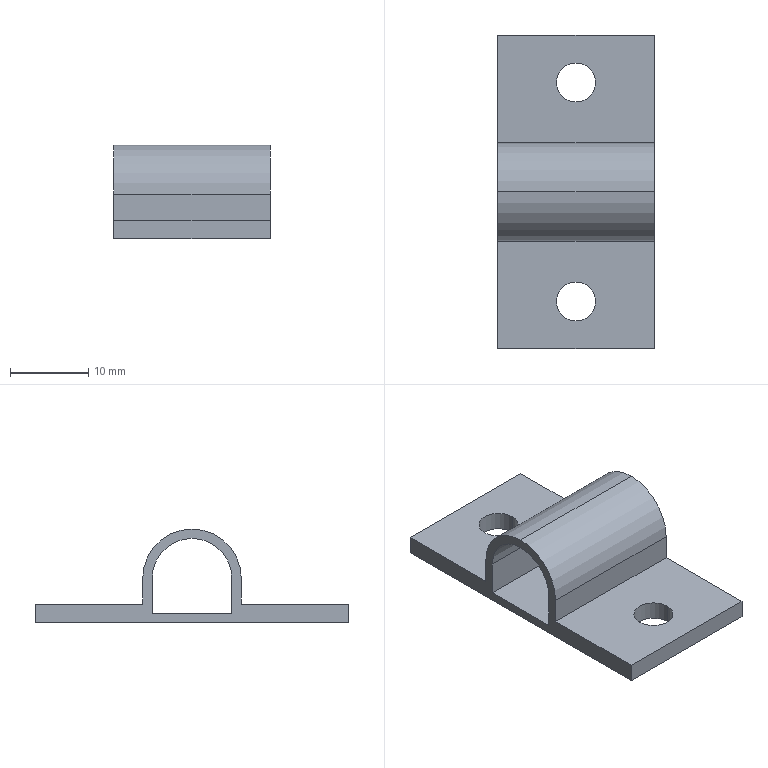Part | SolidWorks | features BaseBody 1 | 1 solid | 20 faces | box 20 x 40 x 12 mm | volume 2169 mm3 | plane 12 | cylinder 8 | commonest cylinder face diameters 5 x4 10.2 x2 12.6 x2
STEP:
#1=CARTESIAN_POINT('',(-7.5,14.,2.4));
#2=VERTEX_POINT('',#1);
#3=CARTESIAN_POINT('',(-12.5,14.,2.4));
#4=VERTEX_POINT('',#3);
#5=CARTESIAN_POINT('',(-10.,14.,2.4));
#6=DIRECTION('',(0.,0.,-1.));
#7=DIRECTION('',(-1.,0.,0.));
#8=AXIS2_PLACEMENT_3D('',#5,#6,#7);
#9=CIRCLE('',#8,2.5);
#10=EDGE_CURVE('',#2,#4,#9,.T.);
#11=ORIENTED_EDGE('',*,*,#10,.F.);
#12=CARTESIAN_POINT('',(-7.5,14.,0.));
#13=VERTEX_POINT('',#12);
#14=CARTESIAN_POINT('',(-7.5,14.,0.));
#15=DIRECTION('',(0.,0.,-1.));
#16=VECTOR('',#15,1000.);
#17=LINE('',#14,#16);
#18=EDGE_CURVE('',#2,#13,#17,.T.);
#19=ORIENTED_EDGE('',*,*,#18,.T.);
#20=CARTESIAN_POINT('',(-12.5,14.,0.));
#21=VERTEX_POINT('',#20);
#22=CARTESIAN_POINT('',(-10.,14.,0.));
#23=DIRECTION('',(0.,0.,1.));
#24=DIRECTION('',(-1.,0.,0.));
#25=AXIS2_PLACEMENT_3D('',#22,#23,#24);
#26=CIRCLE('',#25,2.5);
#27=EDGE_CURVE('',#21,#13,#26,.T.);
#28=ORIENTED_EDGE('',*,*,#27,.F.);
#29=CARTESIAN_POINT('',(-12.5,14.,0.));
#30=DIRECTION('',(0.,0.,-1.));
#31=VECTOR('',#30,1000.);
#32=LINE('',#29,#31);
#33=EDGE_CURVE('',#4,#21,#32,.T.);
#34=ORIENTED_EDGE('',*,*,#33,.F.);
#35=EDGE_LOOP('',(#11,#19,#28,#34));
#36=FACE_OUTER_BOUND('',#35,.T.);
#37=CARTESIAN_POINT('',(-10.,14.,0.));
#38=DIRECTION('',(0.,0.,-1.));
#39=DIRECTION('',(-1.,0.,0.));
#40=AXIS2_PLACEMENT_3D('',#37,#38,#39);
#41=CYLINDRICAL_SURFACE('',#40,2.5);
#42=ADVANCED_FACE('',(#36),#41,.F.);
#43=CARTESIAN_POINT('',(-7.5,-14.,2.4));
#44=VERTEX_POINT('',#43);
#45=CARTESIAN_POINT('',(-12.5,-14.,2.4));
#46=VERTEX_POINT('',#45);
#47=CARTESIAN_POINT('',(-10.,-14.,2.4));
#48=DIRECTION('',(0.,0.,-1.));
#49=DIRECTION('',(-1.,0.,0.));
#50=AXIS2_PLACEMENT_3D('',#47,#48,#49);
#51=CIRCLE('',#50,2.5);
#52=EDGE_CURVE('',#44,#46,#51,.T.);
#53=ORIENTED_EDGE('',*,*,#52,.F.);
#54=CARTESIAN_POINT('',(-7.5,-14.,0.));
#55=VERTEX_POINT('',#54);
#56=CARTESIAN_POINT('',(-7.5,-14.,0.));
#57=DIRECTION('',(0.,0.,-1.));
#58=VECTOR('',#57,1000.);
#59=LINE('',#56,#58);
#60=EDGE_CURVE('',#44,#55,#59,.T.);
#61=ORIENTED_EDGE('',*,*,#60,.T.);
#62=CARTESIAN_POINT('',(-12.5,-14.,0.));
#63=VERTEX_POINT('',#62);
#64=CARTESIAN_POINT('',(-10.,-14.,0.));
#65=DIRECTION('',(0.,0.,1.));
#66=DIRECTION('',(-1.,0.,0.));
#67=AXIS2_PLACEMENT_3D('',#64,#65,#66);
#68=CIRCLE('',#67,2.5);
#69=EDGE_CURVE('',#63,#55,#68,.T.);
#70=ORIENTED_EDGE('',*,*,#69,.F.);
#71=CARTESIAN_POINT('',(-12.5,-14.,0.));
#72=DIRECTION('',(0.,0.,-1.));
#73=VECTOR('',#72,1000.);
#74=LINE('',#71,#73);
#75=EDGE_CURVE('',#46,#63,#74,.T.);
#76=ORIENTED_EDGE('',*,*,#75,.F.);
#77=EDGE_LOOP('',(#53,#61,#70,#76));
#78=FACE_OUTER_BOUND('',#77,.T.);
#79=CARTESIAN_POINT('',(-10.,-14.,0.));
#80=DIRECTION('',(0.,0.,-1.));
#81=DIRECTION('',(-1.,0.,0.));
#82=AXIS2_PLACEMENT_3D('',#79,#80,#81);
#83=CYLINDRICAL_SURFACE('',#82,2.5);
#84=ADVANCED_FACE('',(#78),#83,.F.);
#85=CARTESIAN_POINT('',(0.,0.,10.8));
#86=VERTEX_POINT('',#85);
#87=CARTESIAN_POINT('',(0.,5.1,5.7));
#88=VERTEX_POINT('',#87);
#89=CARTESIAN_POINT('',(0.,0.,5.7));
#90=DIRECTION('',(-1.,0.,0.));
#91=DIRECTION('',(0.,0.,1.));
#92=AXIS2_PLACEMENT_3D('',#89,#90,#91);
#93=CIRCLE('',#92,5.1);
#94=EDGE_CURVE('',#86,#88,#93,.T.);
#95=ORIENTED_EDGE('',*,*,#94,.F.);
#96=CARTESIAN_POINT('',(-20.,0.,10.8));
#97=VERTEX_POINT('',#96);
#98=CARTESIAN_POINT('',(-20.,0.,10.8));
#99=DIRECTION('',(-1.,0.,0.));
#100=VECTOR('',#99,1000.);
#101=LINE('',#98,#100);
#102=EDGE_CURVE('',#86,#97,#101,.T.);
#103=ORIENTED_EDGE('',*,*,#102,.T.);
#104=CARTESIAN_POINT('',(-20.,5.1,5.7));
#105=VERTEX_POINT('',#104);
#106=CARTESIAN_POINT('',(-20.,0.,5.7));
#107=DIRECTION('',(-1.,0.,0.));
#108=DIRECTION('',(0.,0.,1.));
#109=AXIS2_PLACEMENT_3D('',#106,#107,#108);
#110=CIRCLE('',#109,5.1);
#111=EDGE_CURVE('',#97,#105,#110,.T.);
#112=ORIENTED_EDGE('',*,*,#111,.T.);
#113=CARTESIAN_POINT('',(-20.,5.1,5.7));
#114=DIRECTION('',(-1.,0.,0.));
#115=VECTOR('',#114,1000.);
#116=LINE('',#113,#115);
#117=EDGE_CURVE('',#88,#105,#116,.T.);
#118=ORIENTED_EDGE('',*,*,#117,.F.);
#119=EDGE_LOOP('',(#95,#103,#112,#118));
#120=FACE_OUTER_BOUND('',#119,.T.);
#121=CARTESIAN_POINT('',(-20.,0.,5.7));
#122=DIRECTION('',(-1.,0.,0.));
#123=DIRECTION('',(0.,0.,1.));
#124=AXIS2_PLACEMENT_3D('',#121,#122,#123);
#125=CYLINDRICAL_SURFACE('',#124,5.1);
#126=ADVANCED_FACE('',(#120),#125,.F.);
#127=CARTESIAN_POINT('',(0.,0.,12.));
#128=VERTEX_POINT('',#127);
#129=CARTESIAN_POINT('',(0.,-6.3,5.7));
#130=VERTEX_POINT('',#129);
#131=CARTESIAN_POINT('',(0.,0.,5.7));
#132=DIRECTION('',(1.,0.,0.));
#133=DIRECTION('',(0.,0.,1.));
#134=AXIS2_PLACEMENT_3D('',#131,#132,#133);
#135=CIRCLE('',#134,6.3);
#136=EDGE_CURVE('',#128,#130,#135,.T.);
#137=ORIENTED_EDGE('',*,*,#136,.F.);
#138=CARTESIAN_POINT('',(-20.,0.,12.));
#139=VERTEX_POINT('',#138);
#140=CARTESIAN_POINT('',(-20.,0.,12.));
#141=DIRECTION('',(-1.,0.,0.));
#142=VECTOR('',#141,1000.);
#143=LINE('',#140,#142);
#144=EDGE_CURVE('',#128,#139,#143,.T.);
#145=ORIENTED_EDGE('',*,*,#144,.T.);
#146=CARTESIAN_POINT('',(-20.,-6.3,5.7));
#147=VERTEX_POINT('',#146);
#148=CARTESIAN_POINT('',(-20.,0.,5.7));
#149=DIRECTION('',(1.,0.,0.));
#150=DIRECTION('',(0.,0.,1.));
#151=AXIS2_PLACEMENT_3D('',#148,#149,#150);
#152=CIRCLE('',#151,6.3);
#153=EDGE_CURVE('',#139,#147,#152,.T.);
#154=ORIENTED_EDGE('',*,*,#153,.T.);
#155=CARTESIAN_POINT('',(-20.,-6.3,5.7));
#156=DIRECTION('',(1.,0.,0.));
#157=VECTOR('',#156,1000.);
#158=LINE('',#155,#157);
#159=EDGE_CURVE('',#147,#130,#158,.T.);
#160=ORIENTED_EDGE('',*,*,#159,.T.);
#161=EDGE_LOOP('',(#137,#145,#154,#160));
#162=FACE_OUTER_BOUND('',#161,.T.);
#163=CARTESIAN_POINT('',(-20.,0.,5.7));
#164=DIRECTION('',(-1.,0.,0.));
#165=DIRECTION('',(0.,0.,1.));
#166=AXIS2_PLACEMENT_3D('',#163,#164,#165);
#167=CYLINDRICAL_SURFACE('',#166,6.3);
#168=ADVANCED_FACE('',(#162),#167,.T.);
#169=CARTESIAN_POINT('',(-20.,-6.3,2.4));
#170=VERTEX_POINT('',#169);
#171=CARTESIAN_POINT('',(-20.,-6.3,0.));
#172=DIRECTION('',(0.,0.,-1.));
#173=VECTOR('',#172,1000.);
#174=LINE('',#171,#173);
#175=EDGE_CURVE('',#147,#170,#174,.T.);
#176=ORIENTED_EDGE('',*,*,#175,.T.);
#177=CARTESIAN_POINT('',(0.,-6.3,2.4));
#178=VERTEX_POINT('',#177);
#179=CARTESIAN_POINT('',(-20.,-6.3,2.4));
#180=DIRECTION('',(-1.,0.,0.));
#181=VECTOR('',#180,1000.);
#182=LINE('',#179,#181);
#183=EDGE_CURVE('',#178,#170,#182,.T.);
#184=ORIENTED_EDGE('',*,*,#183,.F.);
#185=CARTESIAN_POINT('',(0.,-6.3,0.));
#186=DIRECTION('',(0.,0.,-1.));
#187=VECTOR('',#186,1000.);
#188=LINE('',#185,#187);
#189=EDGE_CURVE('',#130,#178,#188,.T.);
#190=ORIENTED_EDGE('',*,*,#189,.F.);
#191=ORIENTED_EDGE('',*,*,#159,.F.);
#192=EDGE_LOOP('',(#176,#184,#190,#191));
#193=FACE_OUTER_BOUND('',#192,.T.);
#194=CARTESIAN_POINT('',(-20.,-6.3,2.4));
#195=DIRECTION('',(0.,-1.,0.));
#196=DIRECTION('',(0.,0.,-1.));
#197=AXIS2_PLACEMENT_3D('',#194,#195,#196);
#198=PLANE('',#197);
#199=ADVANCED_FACE('',(#193),#198,.T.);
#200=CARTESIAN_POINT('',(-10.,-14.,2.4));
#201=DIRECTION('',(0.,0.,-1.));
#202=DIRECTION('',(-1.,0.,0.));
#203=AXIS2_PLACEMENT_3D('',#200,#201,#202);
#204=CIRCLE('',#203,2.5);
#205=EDGE_CURVE('',#46,#44,#204,.T.);
#206=ORIENTED_EDGE('',*,*,#205,.T.);
#207=ORIENTED_EDGE('',*,*,#52,.T.);
#208=EDGE_LOOP('',(#206,#207));
#209=FACE_BOUND('',#208,.T.);
#210=CARTESIAN_POINT('',(-20.,-20.,2.4));
#211=VERTEX_POINT('',#210);
#212=CARTESIAN_POINT('',(-20.,0.,2.4));
#213=DIRECTION('',(0.,-1.,0.));
#214=VECTOR('',#213,1000.);
#215=LINE('',#212,#214);
#216=EDGE_CURVE('',#170,#211,#215,.T.);
#217=ORIENTED_EDGE('',*,*,#216,.T.);
#218=CARTESIAN_POINT('',(0.,-20.,2.4));
#219=VERTEX_POINT('',#218);
#220=CARTESIAN_POINT('',(-20.,-20.,2.4));
#221=DIRECTION('',(-1.,0.,0.));
#222=VECTOR('',#221,1000.);
#223=LINE('',#220,#222);
#224=EDGE_CURVE('',#219,#211,#223,.T.);
#225=ORIENTED_EDGE('',*,*,#224,.F.);
#226=CARTESIAN_POINT('',(0.,0.,2.4));
#227=DIRECTION('',(0.,-1.,0.));
#228=VECTOR('',#227,1000.);
#229=LINE('',#226,#228);
#230=EDGE_CURVE('',#178,#219,#229,.T.);
#231=ORIENTED_EDGE('',*,*,#230,.F.);
#232=ORIENTED_EDGE('',*,*,#183,.T.);
#233=EDGE_LOOP('',(#217,#225,#231,#232));
#234=FACE_OUTER_BOUND('',#233,.T.);
#235=CARTESIAN_POINT('',(-20.,-20.,2.4));
#236=DIRECTION('',(0.,0.,1.));
#237=DIRECTION('',(0.,-1.,0.));
#238=AXIS2_PLACEMENT_3D('',#235,#236,#237);
#239=PLANE('',#238);
#240=ADVANCED_FACE('',(#209,#234),#239,.T.);
#241=CARTESIAN_POINT('',(-20.,6.3,2.4));
#242=VERTEX_POINT('',#241);
#243=CARTESIAN_POINT('',(-20.,6.3,5.7));
#244=VERTEX_POINT('',#243);
#245=CARTESIAN_POINT('',(-20.,6.3,0.));
#246=DIRECTION('',(0.,0.,1.));
#247=VECTOR('',#246,1000.);
#248=LINE('',#245,#247);
#249=EDGE_CURVE('',#242,#244,#248,.T.);
#250=ORIENTED_EDGE('',*,*,#249,.T.);
#251=CARTESIAN_POINT('',(0.,6.3,5.7));
#252=VERTEX_POINT('',#251);
#253=CARTESIAN_POINT('',(-20.,6.3,5.7));
#254=DIRECTION('',(-1.,0.,0.));
#255=VECTOR('',#254,1000.);
#256=LINE('',#253,#255);
#257=EDGE_CURVE('',#252,#244,#256,.T.);
#258=ORIENTED_EDGE('',*,*,#257,.F.);
#259=CARTESIAN_POINT('',(0.,6.3,2.4));
#260=VERTEX_POINT('',#259);
#261=CARTESIAN_POINT('',(0.,6.3,0.));
#262=DIRECTION('',(0.,0.,1.));
#263=VECTOR('',#262,1000.);
#264=LINE('',#261,#263);
#265=EDGE_CURVE('',#260,#252,#264,.T.);
#266=ORIENTED_EDGE('',*,*,#265,.F.);
#267=CARTESIAN_POINT('',(-20.,6.3,2.4));
#268=DIRECTION('',(1.,0.,0.));
#269=VECTOR('',#268,1000.);
#270=LINE('',#267,#269);
#271=EDGE_CURVE('',#242,#260,#270,.T.);
#272=ORIENTED_EDGE('',*,*,#271,.F.);
#273=EDGE_LOOP('',(#250,#258,#266,#272));
#274=FACE_OUTER_BOUND('',#273,.T.);
#275=CARTESIAN_POINT('',(-20.,6.3,5.7));
#276=DIRECTION('',(0.,1.,0.));
#277=DIRECTION('',(1.,0.,0.));
#278=AXIS2_PLACEMENT_3D('',#275,#276,#277);
#279=PLANE('',#278);
#280=ADVANCED_FACE('',(#274),#279,.T.);
#281=CARTESIAN_POINT('',(-20.,5.1,1.2));
#282=VERTEX_POINT('',#281);
#283=CARTESIAN_POINT('',(-20.,-5.1,1.2));
#284=VERTEX_POINT('',#283);
#285=CARTESIAN_POINT('',(-20.,0.,1.2));
#286=DIRECTION('',(0.,-1.,0.));
#287=VECTOR('',#286,1000.);
#288=LINE('',#285,#287);
#289=EDGE_CURVE('',#282,#284,#288,.T.);
#290=ORIENTED_EDGE('',*,*,#289,.T.);
#291=CARTESIAN_POINT('',(0.,-5.1,1.2));
#292=VERTEX_POINT('',#291);
#293=CARTESIAN_POINT('',(-20.,-5.1,1.2));
#294=DIRECTION('',(-1.,0.,0.));
#295=VECTOR('',#294,1000.);
#296=LINE('',#293,#295);
#297=EDGE_CURVE('',#292,#284,#296,.T.);
#298=ORIENTED_EDGE('',*,*,#297,.F.);
#299=CARTESIAN_POINT('',(0.,5.1,1.2));
#300=VERTEX_POINT('',#299);
#301=CARTESIAN_POINT('',(0.,0.,1.2));
#302=DIRECTION('',(0.,-1.,0.));
#303=VECTOR('',#302,1000.);
#304=LINE('',#301,#303);
#305=EDGE_CURVE('',#300,#292,#304,.T.);
#306=ORIENTED_EDGE('',*,*,#305,.F.);
#307=CARTESIAN_POINT('',(-20.,5.1,1.2));
#308=DIRECTION('',(1.,0.,0.));
#309=VECTOR('',#308,1000.);
#310=LINE('',#307,#309);
#311=EDGE_CURVE('',#282,#300,#310,.T.);
#312=ORIENTED_EDGE('',*,*,#311,.F.);
#313=EDGE_LOOP('',(#290,#298,#306,#312));
#314=FACE_OUTER_BOUND('',#313,.T.);
#315=CARTESIAN_POINT('',(-20.,-5.1,1.2));
#316=DIRECTION('',(0.,0.,1.));
#317=DIRECTION('',(0.,-1.,0.));
#318=AXIS2_PLACEMENT_3D('',#315,#316,#317);
#319=PLANE('',#318);
#320=ADVANCED_FACE('',(#314),#319,.T.);
#321=CARTESIAN_POINT('',(-20.,-5.1,5.7));
#322=VERTEX_POINT('',#321);
#323=CARTESIAN_POINT('',(-20.,-5.1,0.));
#324=DIRECTION('',(0.,0.,1.));
#325=VECTOR('',#324,1000.);
#326=LINE('',#323,#325);
#327=EDGE_CURVE('',#284,#322,#326,.T.);
#328=ORIENTED_EDGE('',*,*,#327,.T.);
#329=CARTESIAN_POINT('',(0.,-5.1,5.7));
#330=VERTEX_POINT('',#329);
#331=CARTESIAN_POINT('',(-20.,-5.1,5.7));
#332=DIRECTION('',(1.,0.,0.));
#333=VECTOR('',#332,1000.);
#334=LINE('',#331,#333);
#335=EDGE_CURVE('',#322,#330,#334,.T.);
#336=ORIENTED_EDGE('',*,*,#335,.T.);
#337=CARTESIAN_POINT('',(0.,-5.1,0.));
#338=DIRECTION('',(0.,0.,1.));
#339=VECTOR('',#338,1000.);
#340=LINE('',#337,#339);
#341=EDGE_CURVE('',#292,#330,#340,.T.);
#342=ORIENTED_EDGE('',*,*,#341,.F.);
#343=ORIENTED_EDGE('',*,*,#297,.T.);
#344=EDGE_LOOP('',(#328,#336,#342,#343));
#345=FACE_OUTER_BOUND('',#344,.T.);
#346=CARTESIAN_POINT('',(-20.,-5.1,5.7));
#347=DIRECTION('',(0.,1.,0.));
#348=DIRECTION('',(1.,0.,0.));
#349=AXIS2_PLACEMENT_3D('',#346,#347,#348);
#350=PLANE('',#349);
#351=ADVANCED_FACE('',(#345),#350,.T.);
#352=CARTESIAN_POINT('',(-20.,5.1,0.));
#353=DIRECTION('',(0.,0.,-1.));
#354=VECTOR('',#353,1000.);
#355=LINE('',#352,#354);
#356=EDGE_CURVE('',#105,#282,#355,.T.);
#357=ORIENTED_EDGE('',*,*,#356,.T.);
#358=ORIENTED_EDGE('',*,*,#311,.T.);
#359=CARTESIAN_POINT('',(0.,5.1,0.));
#360=DIRECTION('',(0.,0.,-1.));
#361=VECTOR('',#360,1000.);
#362=LINE('',#359,#361);
#363=EDGE_CURVE('',#88,#300,#362,.T.);
#364=ORIENTED_EDGE('',*,*,#363,.F.);
#365=ORIENTED_EDGE('',*,*,#117,.T.);
#366=EDGE_LOOP('',(#357,#358,#364,#365));
#367=FACE_OUTER_BOUND('',#366,.T.);
#368=CARTESIAN_POINT('',(-20.,5.1,1.2));
#369=DIRECTION('',(0.,-1.,0.));
#370=DIRECTION('',(0.,0.,-1.));
#371=AXIS2_PLACEMENT_3D('',#368,#369,#370);
#372=PLANE('',#371);
#373=ADVANCED_FACE('',(#367),#372,.T.);
#374=CARTESIAN_POINT('',(-10.,14.,2.4));
#375=DIRECTION('',(0.,0.,-1.));
#376=DIRECTION('',(-1.,0.,0.));
#377=AXIS2_PLACEMENT_3D('',#374,#375,#376);
#378=CIRCLE('',#377,2.5);
#379=EDGE_CURVE('',#4,#2,#378,.T.);
#380=ORIENTED_EDGE('',*,*,#379,.T.);
#381=ORIENTED_EDGE('',*,*,#10,.T.);
#382=EDGE_LOOP('',(#380,#381));
#383=FACE_BOUND('',#382,.T.);
#384=CARTESIAN_POINT('',(-20.,20.,2.4));
#385=VERTEX_POINT('',#384);
#386=CARTESIAN_POINT('',(-20.,0.,2.4));
#387=DIRECTION('',(0.,-1.,0.));
#388=VECTOR('',#387,1000.);
#389=LINE('',#386,#388);
#390=EDGE_CURVE('',#385,#242,#389,.T.);
#391=ORIENTED_EDGE('',*,*,#390,.T.);
#392=ORIENTED_EDGE('',*,*,#271,.T.);
#393=CARTESIAN_POINT('',(0.,20.,2.4));
#394=VERTEX_POINT('',#393);
#395=CARTESIAN_POINT('',(0.,0.,2.4));
#396=DIRECTION('',(0.,-1.,0.));
#397=VECTOR('',#396,1000.);
#398=LINE('',#395,#397);
#399=EDGE_CURVE('',#394,#260,#398,.T.);
#400=ORIENTED_EDGE('',*,*,#399,.F.);
#401=CARTESIAN_POINT('',(-20.,20.,2.4));
#402=DIRECTION('',(1.,0.,0.));
#403=VECTOR('',#402,1000.);
#404=LINE('',#401,#403);
#405=EDGE_CURVE('',#385,#394,#404,.T.);
#406=ORIENTED_EDGE('',*,*,#405,.F.);
#407=EDGE_LOOP('',(#391,#392,#400,#406));
#408=FACE_OUTER_BOUND('',#407,.T.);
#409=CARTESIAN_POINT('',(-20.,6.3,2.4));
#410=DIRECTION('',(0.,0.,1.));
#411=DIRECTION('',(0.,-1.,0.));
#412=AXIS2_PLACEMENT_3D('',#409,#410,#411);
#413=PLANE('',#412);
#414=ADVANCED_FACE('',(#383,#408),#413,.T.);
#415=ORIENTED_EDGE('',*,*,#305,.T.);
#416=ORIENTED_EDGE('',*,*,#341,.T.);
#417=CARTESIAN_POINT('',(0.,0.,5.7));
#418=DIRECTION('',(-1.,0.,0.));
#419=DIRECTION('',(0.,0.,1.));
#420=AXIS2_PLACEMENT_3D('',#417,#418,#419);
#421=CIRCLE('',#420,5.1);
#422=EDGE_CURVE('',#330,#86,#421,.T.);
#423=ORIENTED_EDGE('',*,*,#422,.T.);
#424=ORIENTED_EDGE('',*,*,#94,.T.);
#425=ORIENTED_EDGE('',*,*,#363,.T.);
#426=EDGE_LOOP('',(#415,#416,#423,#424,#425));
#427=FACE_BOUND('',#426,.T.);
#428=CARTESIAN_POINT('',(0.,20.,0.));
#429=VERTEX_POINT('',#428);
#430=CARTESIAN_POINT('',(0.,20.,2.4));
#431=DIRECTION('',(0.,0.,-1.));
#432=VECTOR('',#431,1000.);
#433=LINE('',#430,#432);
#434=EDGE_CURVE('',#394,#429,#433,.T.);
#435=ORIENTED_EDGE('',*,*,#434,.F.);
#436=ORIENTED_EDGE('',*,*,#399,.T.);
#437=ORIENTED_EDGE('',*,*,#265,.T.);
#438=CARTESIAN_POINT('',(0.,0.,5.7));
#439=DIRECTION('',(1.,0.,0.));
#440=DIRECTION('',(0.,0.,1.));
#441=AXIS2_PLACEMENT_3D('',#438,#439,#440);
#442=CIRCLE('',#441,6.3);
#443=EDGE_CURVE('',#252,#128,#442,.T.);
#444=ORIENTED_EDGE('',*,*,#443,.T.);
#445=ORIENTED_EDGE('',*,*,#136,.T.);
#446=ORIENTED_EDGE('',*,*,#189,.T.);
#447=ORIENTED_EDGE('',*,*,#230,.T.);
#448=CARTESIAN_POINT('',(0.,-20.,0.));
#449=VERTEX_POINT('',#448);
#450=CARTESIAN_POINT('',(0.,-20.,0.));
#451=DIRECTION('',(0.,0.,1.));
#452=VECTOR('',#451,1000.);
#453=LINE('',#450,#452);
#454=EDGE_CURVE('',#449,#219,#453,.T.);
#455=ORIENTED_EDGE('',*,*,#454,.F.);
#456=CARTESIAN_POINT('',(0.,20.,0.));
#457=DIRECTION('',(0.,-1.,0.));
#458=VECTOR('',#457,1000.);
#459=LINE('',#456,#458);
#460=EDGE_CURVE('',#429,#449,#459,.T.);
#461=ORIENTED_EDGE('',*,*,#460,.F.);
#462=EDGE_LOOP('',(#435,#436,#437,#444,#445,#446,#447,#455,#461));
#463=FACE_OUTER_BOUND('',#462,.T.);
#464=CARTESIAN_POINT('',(0.,0.,0.));
#465=DIRECTION('',(1.,0.,0.));
#466=DIRECTION('',(0.,1.,0.));
#467=AXIS2_PLACEMENT_3D('',#464,#465,#466);
#468=PLANE('',#467);
#469=ADVANCED_FACE('',(#427,#463),#468,.T.);
#470=CARTESIAN_POINT('',(-20.,-20.,0.));
#471=VERTEX_POINT('',#470);
#472=CARTESIAN_POINT('',(-20.,-20.,0.));
#473=DIRECTION('',(0.,0.,-1.));
#474=VECTOR('',#473,1000.);
#475=LINE('',#472,#474);
#476=EDGE_CURVE('',#211,#471,#475,.T.);
#477=ORIENTED_EDGE('',*,*,#476,.T.);
#478=CARTESIAN_POINT('',(-20.,-20.,0.));
#479=DIRECTION('',(-1.,0.,0.));
#480=VECTOR('',#479,1000.);
#481=LINE('',#478,#480);
#482=EDGE_CURVE('',#449,#471,#481,.T.);
#483=ORIENTED_EDGE('',*,*,#482,.F.);
#484=ORIENTED_EDGE('',*,*,#454,.T.);
#485=ORIENTED_EDGE('',*,*,#224,.T.);
#486=EDGE_LOOP('',(#477,#483,#484,#485));
#487=FACE_OUTER_BOUND('',#486,.T.);
#488=CARTESIAN_POINT('',(-20.,-20.,0.));
#489=DIRECTION('',(0.,-1.,0.));
#490=DIRECTION('',(0.,0.,-1.));
#491=AXIS2_PLACEMENT_3D('',#488,#489,#490);
#492=PLANE('',#491);
#493=ADVANCED_FACE('',(#487),#492,.T.);
#494=CARTESIAN_POINT('',(-20.,0.,5.7));
#495=DIRECTION('',(-1.,0.,0.));
#496=DIRECTION('',(0.,0.,1.));
#497=AXIS2_PLACEMENT_3D('',#494,#495,#496);
#498=CIRCLE('',#497,5.1);
#499=EDGE_CURVE('',#322,#97,#498,.T.);
#500=ORIENTED_EDGE('',*,*,#499,.F.);
#501=ORIENTED_EDGE('',*,*,#327,.F.);
#502=ORIENTED_EDGE('',*,*,#289,.F.);
#503=ORIENTED_EDGE('',*,*,#356,.F.);
#504=ORIENTED_EDGE('',*,*,#111,.F.);
#505=EDGE_LOOP('',(#500,#501,#502,#503,#504));
#506=FACE_BOUND('',#505,.T.);
#507=ORIENTED_EDGE('',*,*,#249,.F.);
#508=ORIENTED_EDGE('',*,*,#390,.F.);
#509=CARTESIAN_POINT('',(-20.,20.,0.));
#510=VERTEX_POINT('',#509);
#511=CARTESIAN_POINT('',(-20.,20.,2.4));
#512=DIRECTION('',(0.,0.,1.));
#513=VECTOR('',#512,1000.);
#514=LINE('',#511,#513);
#515=EDGE_CURVE('',#510,#385,#514,.T.);
#516=ORIENTED_EDGE('',*,*,#515,.F.);
#517=CARTESIAN_POINT('',(-20.,20.,0.));
#518=DIRECTION('',(0.,1.,0.));
#519=VECTOR('',#518,1000.);
#520=LINE('',#517,#519);
#521=EDGE_CURVE('',#471,#510,#520,.T.);
#522=ORIENTED_EDGE('',*,*,#521,.F.);
#523=ORIENTED_EDGE('',*,*,#476,.F.);
#524=ORIENTED_EDGE('',*,*,#216,.F.);
#525=ORIENTED_EDGE('',*,*,#175,.F.);
#526=ORIENTED_EDGE('',*,*,#153,.F.);
#527=CARTESIAN_POINT('',(-20.,0.,5.7));
#528=DIRECTION('',(1.,0.,0.));
#529=DIRECTION('',(0.,0.,1.));
#530=AXIS2_PLACEMENT_3D('',#527,#528,#529);
#531=CIRCLE('',#530,6.3);
#532=EDGE_CURVE('',#244,#139,#531,.T.);
#533=ORIENTED_EDGE('',*,*,#532,.F.);
#534=EDGE_LOOP('',(#507,#508,#516,#522,#523,#524,#525,#526,#533));
#535=FACE_OUTER_BOUND('',#534,.T.);
#536=CARTESIAN_POINT('',(-20.,0.,0.));
#537=DIRECTION('',(1.,0.,0.));
#538=DIRECTION('',(0.,1.,0.));
#539=AXIS2_PLACEMENT_3D('',#536,#537,#538);
#540=PLANE('',#539);
#541=ADVANCED_FACE('',(#506,#535),#540,.F.);
#542=ORIENTED_EDGE('',*,*,#515,.T.);
#543=ORIENTED_EDGE('',*,*,#405,.T.);
#544=ORIENTED_EDGE('',*,*,#434,.T.);
#545=CARTESIAN_POINT('',(-20.,20.,0.));
#546=DIRECTION('',(1.,0.,0.));
#547=VECTOR('',#546,1000.);
#548=LINE('',#545,#547);
#549=EDGE_CURVE('',#510,#429,#548,.T.);
#550=ORIENTED_EDGE('',*,*,#549,.F.);
#551=EDGE_LOOP('',(#542,#543,#544,#550));
#552=FACE_OUTER_BOUND('',#551,.T.);
#553=CARTESIAN_POINT('',(-20.,20.,2.4));
#554=DIRECTION('',(0.,1.,0.));
#555=DIRECTION('',(1.,0.,0.));
#556=AXIS2_PLACEMENT_3D('',#553,#554,#555);
#557=PLANE('',#556);
#558=ADVANCED_FACE('',(#552),#557,.T.);
#559=ORIENTED_EDGE('',*,*,#69,.T.);
#560=CARTESIAN_POINT('',(-10.,-14.,0.));
#561=DIRECTION('',(0.,0.,1.));
#562=DIRECTION('',(-1.,0.,0.));
#563=AXIS2_PLACEMENT_3D('',#560,#561,#562);
#564=CIRCLE('',#563,2.5);
#565=EDGE_CURVE('',#55,#63,#564,.T.);
#566=ORIENTED_EDGE('',*,*,#565,.T.);
#567=EDGE_LOOP('',(#559,#566));
#568=FACE_BOUND('',#567,.T.);
#569=ORIENTED_EDGE('',*,*,#27,.T.);
#570=CARTESIAN_POINT('',(-10.,14.,0.));
#571=DIRECTION('',(0.,0.,1.));
#572=DIRECTION('',(-1.,0.,0.));
#573=AXIS2_PLACEMENT_3D('',#570,#571,#572);
#574=CIRCLE('',#573,2.5);
#575=EDGE_CURVE('',#13,#21,#574,.T.);
#576=ORIENTED_EDGE('',*,*,#575,.T.);
#577=EDGE_LOOP('',(#569,#576));
#578=FACE_BOUND('',#577,.T.);
#579=ORIENTED_EDGE('',*,*,#521,.T.);
#580=ORIENTED_EDGE('',*,*,#549,.T.);
#581=ORIENTED_EDGE('',*,*,#460,.T.);
#582=ORIENTED_EDGE('',*,*,#482,.T.);
#583=EDGE_LOOP('',(#579,#580,#581,#582));
#584=FACE_OUTER_BOUND('',#583,.T.);
#585=CARTESIAN_POINT('',(-20.,20.,0.));
#586=DIRECTION('',(0.,0.,-1.));
#587=DIRECTION('',(0.,-1.,0.));
#588=AXIS2_PLACEMENT_3D('',#585,#586,#587);
#589=PLANE('',#588);
#590=ADVANCED_FACE('',(#568,#578,#584),#589,.T.);
#591=ORIENTED_EDGE('',*,*,#144,.F.);
#592=ORIENTED_EDGE('',*,*,#443,.F.);
#593=ORIENTED_EDGE('',*,*,#257,.T.);
#594=ORIENTED_EDGE('',*,*,#532,.T.);
#595=EDGE_LOOP('',(#591,#592,#593,#594));
#596=FACE_OUTER_BOUND('',#595,.T.);
#597=CARTESIAN_POINT('',(-20.,0.,5.7));
#598=DIRECTION('',(-1.,0.,0.));
#599=DIRECTION('',(0.,0.,1.));
#600=AXIS2_PLACEMENT_3D('',#597,#598,#599);
#601=CYLINDRICAL_SURFACE('',#600,6.3);
#602=ADVANCED_FACE('',(#596),#601,.T.);
#603=ORIENTED_EDGE('',*,*,#102,.F.);
#604=ORIENTED_EDGE('',*,*,#422,.F.);
#605=ORIENTED_EDGE('',*,*,#335,.F.);
#606=ORIENTED_EDGE('',*,*,#499,.T.);
#607=EDGE_LOOP('',(#603,#604,#605,#606));
#608=FACE_OUTER_BOUND('',#607,.T.);
#609=CARTESIAN_POINT('',(-20.,0.,5.7));
#610=DIRECTION('',(-1.,0.,0.));
#611=DIRECTION('',(0.,0.,1.));
#612=AXIS2_PLACEMENT_3D('',#609,#610,#611);
#613=CYLINDRICAL_SURFACE('',#612,5.1);
#614=ADVANCED_FACE('',(#608),#613,.F.);
#615=ORIENTED_EDGE('',*,*,#60,.F.);
#616=ORIENTED_EDGE('',*,*,#205,.F.);
#617=ORIENTED_EDGE('',*,*,#75,.T.);
#618=ORIENTED_EDGE('',*,*,#565,.F.);
#619=EDGE_LOOP('',(#615,#616,#617,#618));
#620=FACE_OUTER_BOUND('',#619,.T.);
#621=CARTESIAN_POINT('',(-10.,-14.,0.));
#622=DIRECTION('',(0.,0.,-1.));
#623=DIRECTION('',(-1.,0.,0.));
#624=AXIS2_PLACEMENT_3D('',#621,#622,#623);
#625=CYLINDRICAL_SURFACE('',#624,2.5);
#626=ADVANCED_FACE('',(#620),#625,.F.);
#627=ORIENTED_EDGE('',*,*,#18,.F.);
#628=ORIENTED_EDGE('',*,*,#379,.F.);
#629=ORIENTED_EDGE('',*,*,#33,.T.);
#630=ORIENTED_EDGE('',*,*,#575,.F.);
#631=EDGE_LOOP('',(#627,#628,#629,#630));
#632=FACE_OUTER_BOUND('',#631,.T.);
#633=CARTESIAN_POINT('',(-10.,14.,0.));
#634=DIRECTION('',(0.,0.,-1.));
#635=DIRECTION('',(-1.,0.,0.));
#636=AXIS2_PLACEMENT_3D('',#633,#634,#635);
#637=CYLINDRICAL_SURFACE('',#636,2.5);
#638=ADVANCED_FACE('',(#632),#637,.F.);
#639=CLOSED_SHELL('',(#42,#84,#126,#168,#199,#240,#280,#320,#351,#373,#414,#469,#493,#541,#558,#590,#602,#614,#626,#638));
#640=MANIFOLD_SOLID_BREP('',#639);
#641=CARTESIAN_POINT('',(0.,0.,0.));
#642=DIRECTION('',(0.,0.,1.));
#643=DIRECTION('',(1.,0.,0.));
#644=AXIS2_PLACEMENT_3D('',#641,#642,#643);
#645=(LENGTH_UNIT()NAMED_UNIT(*)SI_UNIT(.MILLI.,.METRE.));
#646=UNCERTAINTY_MEASURE_WITH_UNIT(LENGTH_MEASURE(0.00001),#645,'','');
#647=(NAMED_UNIT(*)PLANE_ANGLE_UNIT()SI_UNIT($,.RADIAN.));
#648=(NAMED_UNIT(*)SI_UNIT($,.STERADIAN.)SOLID_ANGLE_UNIT());
#649=(GEOMETRIC_REPRESENTATION_CONTEXT(3)GLOBAL_UNCERTAINTY_ASSIGNED_CONTEXT((#646))GLOBAL_UNIT_ASSIGNED_CONTEXT((#645,#647,#648))REPRESENTATION_CONTEXT('',''));
#650=ADVANCED_BREP_SHAPE_REPRESENTATION('',(#640,#644),#649);